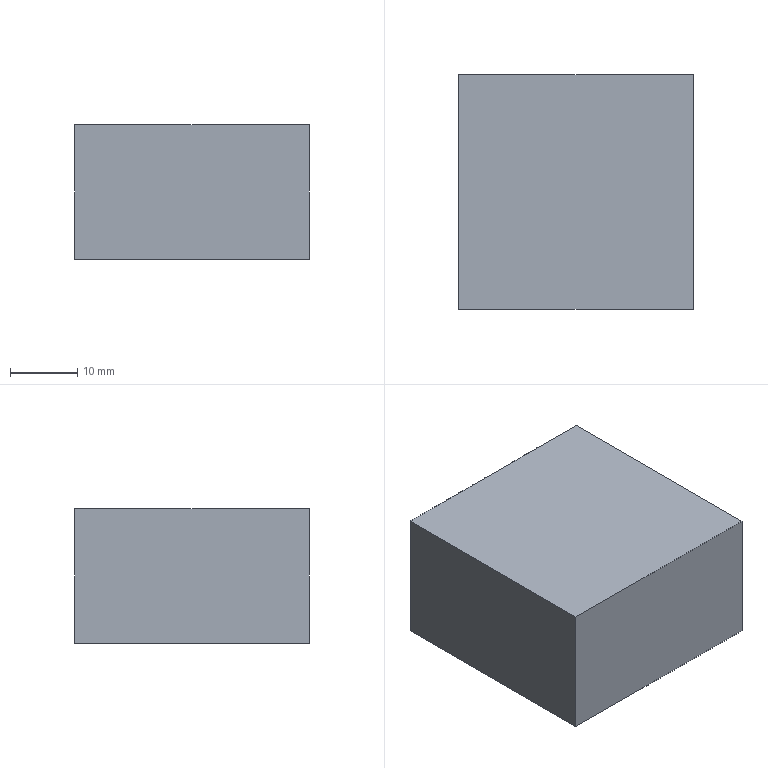Part | SolidWorks | features Extrusion 1, Shell 1 | 1 solid | 11 faces | box 35 x 35 x 20 mm | volume 3809 mm3 | plane 11
STEP:
#1=CARTESIAN_POINT('',(-109.,-4.,0.));
#2=VERTEX_POINT('',#1);
#3=CARTESIAN_POINT('',(-109.,-39.,0.));
#4=VERTEX_POINT('',#3);
#5=CARTESIAN_POINT('',(-109.,-4.,0.));
#6=DIRECTION('',(0.,-1.,0.));
#7=VECTOR('',#6,1000.);
#8=LINE('',#5,#7);
#9=EDGE_CURVE('',#2,#4,#8,.T.);
#10=ORIENTED_EDGE('',*,*,#9,.F.);
#11=CARTESIAN_POINT('',(-109.,-4.,-20.));
#12=VERTEX_POINT('',#11);
#13=CARTESIAN_POINT('',(-109.,-4.,-20.));
#14=DIRECTION('',(0.,0.,1.));
#15=VECTOR('',#14,1000.);
#16=LINE('',#13,#15);
#17=EDGE_CURVE('',#12,#2,#16,.T.);
#18=ORIENTED_EDGE('',*,*,#17,.F.);
#19=CARTESIAN_POINT('',(-109.,-39.,-20.));
#20=VERTEX_POINT('',#19);
#21=CARTESIAN_POINT('',(-109.,-4.,-20.));
#22=DIRECTION('',(0.,-1.,0.));
#23=VECTOR('',#22,1000.);
#24=LINE('',#21,#23);
#25=EDGE_CURVE('',#12,#20,#24,.T.);
#26=ORIENTED_EDGE('',*,*,#25,.T.);
#27=CARTESIAN_POINT('',(-109.,-39.,-20.));
#28=DIRECTION('',(0.,0.,1.));
#29=VECTOR('',#28,1000.);
#30=LINE('',#27,#29);
#31=EDGE_CURVE('',#20,#4,#30,.T.);
#32=ORIENTED_EDGE('',*,*,#31,.T.);
#33=EDGE_LOOP('',(#10,#18,#26,#32));
#34=FACE_OUTER_BOUND('',#33,.T.);
#35=CARTESIAN_POINT('',(-109.,-4.,-20.));
#36=DIRECTION('',(-1.,0.,0.));
#37=DIRECTION('',(0.,0.,1.));
#38=AXIS2_PLACEMENT_3D('',#35,#36,#37);
#39=PLANE('',#38);
#40=ADVANCED_FACE('',(#34),#39,.T.);
#41=CARTESIAN_POINT('',(-74.,-4.,0.));
#42=VERTEX_POINT('',#41);
#43=CARTESIAN_POINT('',(-74.,-4.,0.));
#44=DIRECTION('',(-1.,0.,0.));
#45=VECTOR('',#44,1000.);
#46=LINE('',#43,#45);
#47=EDGE_CURVE('',#42,#2,#46,.T.);
#48=ORIENTED_EDGE('',*,*,#47,.F.);
#49=CARTESIAN_POINT('',(-74.,-4.,-20.));
#50=VERTEX_POINT('',#49);
#51=CARTESIAN_POINT('',(-74.,-4.,-20.));
#52=DIRECTION('',(0.,0.,1.));
#53=VECTOR('',#52,1000.);
#54=LINE('',#51,#53);
#55=EDGE_CURVE('',#50,#42,#54,.T.);
#56=ORIENTED_EDGE('',*,*,#55,.F.);
#57=CARTESIAN_POINT('',(-74.,-4.,-20.));
#58=DIRECTION('',(-1.,0.,0.));
#59=VECTOR('',#58,1000.);
#60=LINE('',#57,#59);
#61=EDGE_CURVE('',#50,#12,#60,.T.);
#62=ORIENTED_EDGE('',*,*,#61,.T.);
#63=ORIENTED_EDGE('',*,*,#17,.T.);
#64=EDGE_LOOP('',(#48,#56,#62,#63));
#65=FACE_OUTER_BOUND('',#64,.T.);
#66=CARTESIAN_POINT('',(-74.,-4.,-20.));
#67=DIRECTION('',(0.,1.,0.));
#68=DIRECTION('',(0.,0.,1.));
#69=AXIS2_PLACEMENT_3D('',#66,#67,#68);
#70=PLANE('',#69);
#71=ADVANCED_FACE('',(#65),#70,.T.);
#72=CARTESIAN_POINT('',(-74.,-39.,0.));
#73=VERTEX_POINT('',#72);
#74=CARTESIAN_POINT('',(-74.,-39.,0.));
#75=DIRECTION('',(0.,1.,0.));
#76=VECTOR('',#75,1000.);
#77=LINE('',#74,#76);
#78=EDGE_CURVE('',#73,#42,#77,.T.);
#79=ORIENTED_EDGE('',*,*,#78,.F.);
#80=CARTESIAN_POINT('',(-74.,-39.,-20.));
#81=VERTEX_POINT('',#80);
#82=CARTESIAN_POINT('',(-74.,-39.,-20.));
#83=DIRECTION('',(0.,0.,1.));
#84=VECTOR('',#83,1000.);
#85=LINE('',#82,#84);
#86=EDGE_CURVE('',#81,#73,#85,.T.);
#87=ORIENTED_EDGE('',*,*,#86,.F.);
#88=CARTESIAN_POINT('',(-74.,-39.,-20.));
#89=DIRECTION('',(0.,1.,0.));
#90=VECTOR('',#89,1000.);
#91=LINE('',#88,#90);
#92=EDGE_CURVE('',#81,#50,#91,.T.);
#93=ORIENTED_EDGE('',*,*,#92,.T.);
#94=ORIENTED_EDGE('',*,*,#55,.T.);
#95=EDGE_LOOP('',(#79,#87,#93,#94));
#96=FACE_OUTER_BOUND('',#95,.T.);
#97=CARTESIAN_POINT('',(-74.,-39.,-20.));
#98=DIRECTION('',(1.,0.,0.));
#99=DIRECTION('',(0.,0.,-1.));
#100=AXIS2_PLACEMENT_3D('',#97,#98,#99);
#101=PLANE('',#100);
#102=ADVANCED_FACE('',(#96),#101,.T.);
#103=CARTESIAN_POINT('',(-109.,-39.,0.));
#104=DIRECTION('',(1.,0.,0.));
#105=VECTOR('',#104,1000.);
#106=LINE('',#103,#105);
#107=EDGE_CURVE('',#4,#73,#106,.T.);
#108=ORIENTED_EDGE('',*,*,#107,.F.);
#109=ORIENTED_EDGE('',*,*,#31,.F.);
#110=CARTESIAN_POINT('',(-109.,-39.,-20.));
#111=DIRECTION('',(1.,0.,0.));
#112=VECTOR('',#111,1000.);
#113=LINE('',#110,#112);
#114=EDGE_CURVE('',#20,#81,#113,.T.);
#115=ORIENTED_EDGE('',*,*,#114,.T.);
#116=ORIENTED_EDGE('',*,*,#86,.T.);
#117=EDGE_LOOP('',(#108,#109,#115,#116));
#118=FACE_OUTER_BOUND('',#117,.T.);
#119=CARTESIAN_POINT('',(-109.,-39.,-20.));
#120=DIRECTION('',(0.,-1.,0.));
#121=DIRECTION('',(0.,0.,-1.));
#122=AXIS2_PLACEMENT_3D('',#119,#120,#121);
#123=PLANE('',#122);
#124=ADVANCED_FACE('',(#118),#123,.T.);
#125=CARTESIAN_POINT('',(-75.,-5.,-20.));
#126=VERTEX_POINT('',#125);
#127=CARTESIAN_POINT('',(-108.,-5.,-20.));
#128=VERTEX_POINT('',#127);
#129=CARTESIAN_POINT('',(0.,-5.,-20.));
#130=DIRECTION('',(-1.,0.,0.));
#131=VECTOR('',#130,1000.);
#132=LINE('',#129,#131);
#133=EDGE_CURVE('',#126,#128,#132,.T.);
#134=ORIENTED_EDGE('',*,*,#133,.T.);
#135=CARTESIAN_POINT('',(-108.,-38.,-20.));
#136=VERTEX_POINT('',#135);
#137=CARTESIAN_POINT('',(-108.,0.,-20.));
#138=DIRECTION('',(0.,-1.,0.));
#139=VECTOR('',#138,1000.);
#140=LINE('',#137,#139);
#141=EDGE_CURVE('',#128,#136,#140,.T.);
#142=ORIENTED_EDGE('',*,*,#141,.T.);
#143=CARTESIAN_POINT('',(-75.,-38.,-20.));
#144=VERTEX_POINT('',#143);
#145=CARTESIAN_POINT('',(0.,-38.,-20.));
#146=DIRECTION('',(1.,0.,0.));
#147=VECTOR('',#146,1000.);
#148=LINE('',#145,#147);
#149=EDGE_CURVE('',#136,#144,#148,.T.);
#150=ORIENTED_EDGE('',*,*,#149,.T.);
#151=CARTESIAN_POINT('',(-75.,0.,-20.));
#152=DIRECTION('',(0.,1.,0.));
#153=VECTOR('',#152,1000.);
#154=LINE('',#151,#153);
#155=EDGE_CURVE('',#144,#126,#154,.T.);
#156=ORIENTED_EDGE('',*,*,#155,.T.);
#157=EDGE_LOOP('',(#134,#142,#150,#156));
#158=FACE_BOUND('',#157,.T.);
#159=ORIENTED_EDGE('',*,*,#25,.F.);
#160=ORIENTED_EDGE('',*,*,#61,.F.);
#161=ORIENTED_EDGE('',*,*,#92,.F.);
#162=ORIENTED_EDGE('',*,*,#114,.F.);
#163=EDGE_LOOP('',(#159,#160,#161,#162));
#164=FACE_OUTER_BOUND('',#163,.T.);
#165=CARTESIAN_POINT('',(0.,0.,-20.));
#166=DIRECTION('',(0.,0.,1.));
#167=DIRECTION('',(1.,0.,0.));
#168=AXIS2_PLACEMENT_3D('',#165,#166,#167);
#169=PLANE('',#168);
#170=ADVANCED_FACE('',(#158,#164),#169,.F.);
#171=ORIENTED_EDGE('',*,*,#9,.T.);
#172=ORIENTED_EDGE('',*,*,#107,.T.);
#173=ORIENTED_EDGE('',*,*,#78,.T.);
#174=ORIENTED_EDGE('',*,*,#47,.T.);
#175=EDGE_LOOP('',(#171,#172,#173,#174));
#176=FACE_OUTER_BOUND('',#175,.T.);
#177=CARTESIAN_POINT('',(0.,0.,0.));
#178=DIRECTION('',(0.,0.,1.));
#179=DIRECTION('',(1.,0.,0.));
#180=AXIS2_PLACEMENT_3D('',#177,#178,#179);
#181=PLANE('',#180);
#182=ADVANCED_FACE('',(#176),#181,.T.);
#183=CARTESIAN_POINT('',(-108.,-5.,-1.));
#184=VERTEX_POINT('',#183);
#185=CARTESIAN_POINT('',(-108.,-38.,-1.));
#186=VERTEX_POINT('',#185);
#187=CARTESIAN_POINT('',(-108.,0.,-1.));
#188=DIRECTION('',(0.,-1.,0.));
#189=VECTOR('',#188,1000.);
#190=LINE('',#187,#189);
#191=EDGE_CURVE('',#184,#186,#190,.T.);
#192=ORIENTED_EDGE('',*,*,#191,.T.);
#193=CARTESIAN_POINT('',(-108.,-38.,-20.));
#194=DIRECTION('',(0.,0.,1.));
#195=VECTOR('',#194,1000.);
#196=LINE('',#193,#195);
#197=EDGE_CURVE('',#136,#186,#196,.T.);
#198=ORIENTED_EDGE('',*,*,#197,.F.);
#199=ORIENTED_EDGE('',*,*,#141,.F.);
#200=CARTESIAN_POINT('',(-108.,-5.,-20.));
#201=DIRECTION('',(0.,0.,1.));
#202=VECTOR('',#201,1000.);
#203=LINE('',#200,#202);
#204=EDGE_CURVE('',#128,#184,#203,.T.);
#205=ORIENTED_EDGE('',*,*,#204,.T.);
#206=EDGE_LOOP('',(#192,#198,#199,#205));
#207=FACE_OUTER_BOUND('',#206,.T.);
#208=CARTESIAN_POINT('',(-108.,-4.,-20.));
#209=DIRECTION('',(-1.,0.,0.));
#210=DIRECTION('',(0.,0.,1.));
#211=AXIS2_PLACEMENT_3D('',#208,#209,#210);
#212=PLANE('',#211);
#213=ADVANCED_FACE('',(#207),#212,.F.);
#214=CARTESIAN_POINT('',(-75.,-5.,-1.));
#215=VERTEX_POINT('',#214);
#216=CARTESIAN_POINT('',(0.,-5.,-1.));
#217=DIRECTION('',(-1.,0.,0.));
#218=VECTOR('',#217,1000.);
#219=LINE('',#216,#218);
#220=EDGE_CURVE('',#215,#184,#219,.T.);
#221=ORIENTED_EDGE('',*,*,#220,.T.);
#222=ORIENTED_EDGE('',*,*,#204,.F.);
#223=ORIENTED_EDGE('',*,*,#133,.F.);
#224=CARTESIAN_POINT('',(-75.,-5.,-20.));
#225=DIRECTION('',(0.,0.,1.));
#226=VECTOR('',#225,1000.);
#227=LINE('',#224,#226);
#228=EDGE_CURVE('',#126,#215,#227,.T.);
#229=ORIENTED_EDGE('',*,*,#228,.T.);
#230=EDGE_LOOP('',(#221,#222,#223,#229));
#231=FACE_OUTER_BOUND('',#230,.T.);
#232=CARTESIAN_POINT('',(-74.,-5.,-20.));
#233=DIRECTION('',(0.,1.,0.));
#234=DIRECTION('',(0.,0.,1.));
#235=AXIS2_PLACEMENT_3D('',#232,#233,#234);
#236=PLANE('',#235);
#237=ADVANCED_FACE('',(#231),#236,.F.);
#238=CARTESIAN_POINT('',(-75.,-38.,-1.));
#239=VERTEX_POINT('',#238);
#240=CARTESIAN_POINT('',(-75.,0.,-1.));
#241=DIRECTION('',(0.,1.,0.));
#242=VECTOR('',#241,1000.);
#243=LINE('',#240,#242);
#244=EDGE_CURVE('',#239,#215,#243,.T.);
#245=ORIENTED_EDGE('',*,*,#244,.T.);
#246=ORIENTED_EDGE('',*,*,#228,.F.);
#247=ORIENTED_EDGE('',*,*,#155,.F.);
#248=CARTESIAN_POINT('',(-75.,-38.,-20.));
#249=DIRECTION('',(0.,0.,1.));
#250=VECTOR('',#249,1000.);
#251=LINE('',#248,#250);
#252=EDGE_CURVE('',#144,#239,#251,.T.);
#253=ORIENTED_EDGE('',*,*,#252,.T.);
#254=EDGE_LOOP('',(#245,#246,#247,#253));
#255=FACE_OUTER_BOUND('',#254,.T.);
#256=CARTESIAN_POINT('',(-75.,-39.,-20.));
#257=DIRECTION('',(1.,0.,0.));
#258=DIRECTION('',(0.,0.,-1.));
#259=AXIS2_PLACEMENT_3D('',#256,#257,#258);
#260=PLANE('',#259);
#261=ADVANCED_FACE('',(#255),#260,.F.);
#262=CARTESIAN_POINT('',(0.,-38.,-1.));
#263=DIRECTION('',(1.,0.,0.));
#264=VECTOR('',#263,1000.);
#265=LINE('',#262,#264);
#266=EDGE_CURVE('',#186,#239,#265,.T.);
#267=ORIENTED_EDGE('',*,*,#266,.T.);
#268=ORIENTED_EDGE('',*,*,#252,.F.);
#269=ORIENTED_EDGE('',*,*,#149,.F.);
#270=ORIENTED_EDGE('',*,*,#197,.T.);
#271=EDGE_LOOP('',(#267,#268,#269,#270));
#272=FACE_OUTER_BOUND('',#271,.T.);
#273=CARTESIAN_POINT('',(-109.,-38.,-20.));
#274=DIRECTION('',(0.,-1.,0.));
#275=DIRECTION('',(0.,0.,-1.));
#276=AXIS2_PLACEMENT_3D('',#273,#274,#275);
#277=PLANE('',#276);
#278=ADVANCED_FACE('',(#272),#277,.F.);
#279=ORIENTED_EDGE('',*,*,#191,.F.);
#280=ORIENTED_EDGE('',*,*,#220,.F.);
#281=ORIENTED_EDGE('',*,*,#244,.F.);
#282=ORIENTED_EDGE('',*,*,#266,.F.);
#283=EDGE_LOOP('',(#279,#280,#281,#282));
#284=FACE_OUTER_BOUND('',#283,.T.);
#285=CARTESIAN_POINT('',(0.,0.,-1.));
#286=DIRECTION('',(0.,0.,1.));
#287=DIRECTION('',(1.,0.,0.));
#288=AXIS2_PLACEMENT_3D('',#285,#286,#287);
#289=PLANE('',#288);
#290=ADVANCED_FACE('',(#284),#289,.F.);
#291=CLOSED_SHELL('',(#40,#71,#102,#124,#170,#182,#213,#237,#261,#278,#290));
#292=MANIFOLD_SOLID_BREP('',#291);
#293=CARTESIAN_POINT('',(0.,0.,0.));
#294=DIRECTION('',(0.,0.,1.));
#295=DIRECTION('',(1.,0.,0.));
#296=AXIS2_PLACEMENT_3D('',#293,#294,#295);
#297=(LENGTH_UNIT()NAMED_UNIT(*)SI_UNIT(.MILLI.,.METRE.));
#298=UNCERTAINTY_MEASURE_WITH_UNIT(LENGTH_MEASURE(0.00001),#297,'','');
#299=(NAMED_UNIT(*)PLANE_ANGLE_UNIT()SI_UNIT($,.RADIAN.));
#300=(NAMED_UNIT(*)SI_UNIT($,.STERADIAN.)SOLID_ANGLE_UNIT());
#301=(GEOMETRIC_REPRESENTATION_CONTEXT(3)GLOBAL_UNCERTAINTY_ASSIGNED_CONTEXT((#298))GLOBAL_UNIT_ASSIGNED_CONTEXT((#297,#299,#300))REPRESENTATION_CONTEXT('',''));
#302=ADVANCED_BREP_SHAPE_REPRESENTATION('',(#292,#296),#301);